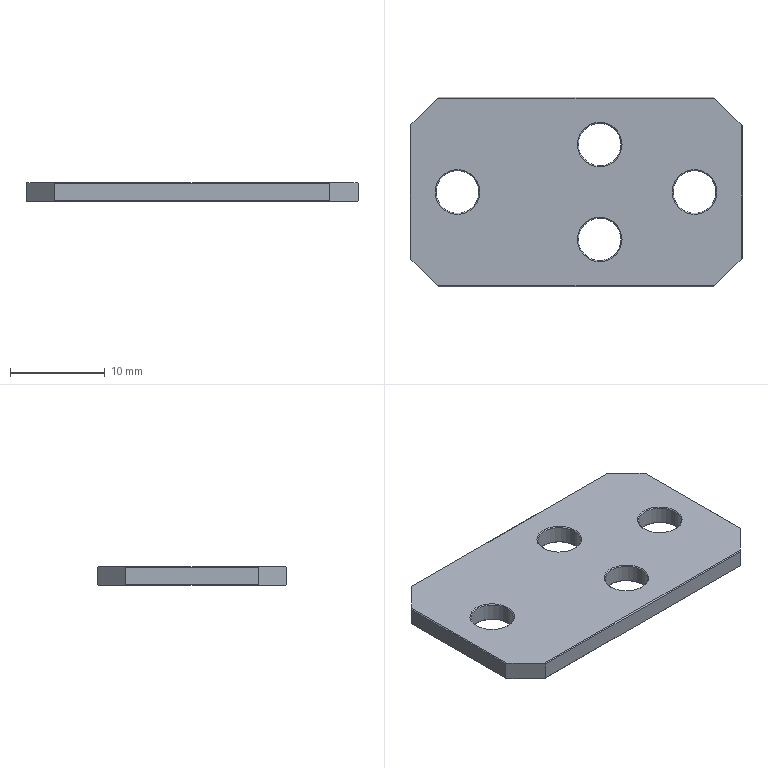Part | STEP file | Photo seat | 1 solid | 42 faces | box 35 x 20 x 2 mm | volume 1235 mm3 | plane 18 | cone 16 | cylinder 8 | commonest cylinder face diameters 4.5 x8